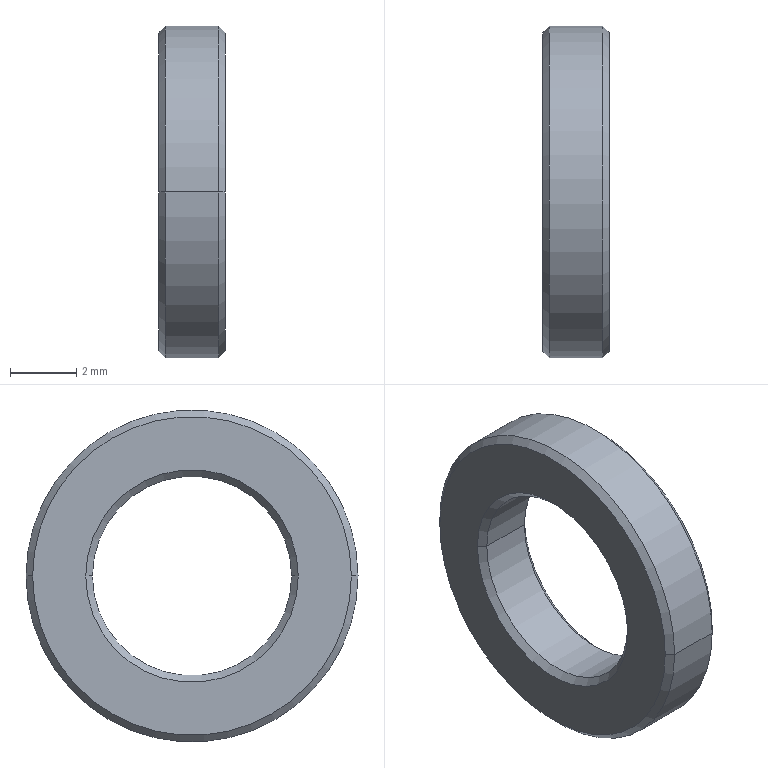Part | STEP file | WSSS10-6-2-32 | 1 solid | 14 faces | box 2 x 10 x 10 mm | volume 98.52 mm3 | cone 8 | cylinder 4 | plane 2 | commonest cylinder face diameters 6 x2 10 x2
STEP:
#1=CARTESIAN_POINT('',(0.,0.,0.));
#2=DIRECTION('',(0.,0.,1.));
#3=DIRECTION('',(1.,0.,0.));
#4=AXIS2_PLACEMENT_3D('',#1,#2,#3);
#5=CARTESIAN_POINT('',(1.8,-3.,0.));
#6=VERTEX_POINT('',#5);
#7=CARTESIAN_POINT('',(0.2,-3.,0.));
#8=VERTEX_POINT('',#7);
#9=CARTESIAN_POINT('',(-3.,-3.,0.));
#10=DIRECTION('',(-1.,0.,0.));
#11=VECTOR('',#10,1.);
#12=LINE('',#9,#11);
#13=CARTESIAN_POINT('',(-3.,0.,0.));
#14=DIRECTION('',(-1.,0.,0.));
#15=DIRECTION('',(0.,-1.,0.));
#16=AXIS2_PLACEMENT_3D('',#13,#14,#15);
#17=CYLINDRICAL_SURFACE('',#16,3.);
#18=CARTESIAN_POINT('',(6.283,0.));
#19=DIRECTION('',(0.,1.));
#20=VECTOR('',#19,1.);
#21=LINE('',#18,#20);
#22=(GEOMETRIC_REPRESENTATION_CONTEXT(2)PARAMETRIC_REPRESENTATION_CONTEXT()REPRESENTATION_CONTEXT('',''));
#23=DEFINITIONAL_REPRESENTATION('',(#21),#22);
#24=PCURVE('',#17,#23);
#25=CARTESIAN_POINT('',(-3.,0.,0.));
#26=DIRECTION('',(-1.,0.,0.));
#27=DIRECTION('',(0.,-1.,0.));
#28=AXIS2_PLACEMENT_3D('',#25,#26,#27);
#29=CYLINDRICAL_SURFACE('',#28,3.);
#30=CARTESIAN_POINT('',(0.,0.));
#31=DIRECTION('',(0.,1.));
#32=VECTOR('',#31,1.);
#33=LINE('',#30,#32);
#34=(GEOMETRIC_REPRESENTATION_CONTEXT(2)PARAMETRIC_REPRESENTATION_CONTEXT()REPRESENTATION_CONTEXT('',''));
#35=DEFINITIONAL_REPRESENTATION('',(#33),#34);
#36=PCURVE('',#29,#35);
#37=SURFACE_CURVE('',#12,(#24,#36),.PCURVE_S1.);
#38=EDGE_CURVE('',#6,#8,#37,.T.);
#39=ORIENTED_EDGE('',*,*,#38,.T.);
#40=CARTESIAN_POINT('',(0.2,3.,0.));
#41=VERTEX_POINT('',#40);
#42=CARTESIAN_POINT('',(0.2,0.,0.));
#43=DIRECTION('',(-1.,0.,0.));
#44=DIRECTION('',(0.,-1.,0.));
#45=AXIS2_PLACEMENT_3D('',#42,#43,#44);
#46=CIRCLE('',#45,3.);
#47=CARTESIAN_POINT('',(0.,-3.2));
#48=DIRECTION('',(1.,0.));
#49=VECTOR('',#48,1.);
#50=LINE('',#47,#49);
#51=(GEOMETRIC_REPRESENTATION_CONTEXT(2)PARAMETRIC_REPRESENTATION_CONTEXT()REPRESENTATION_CONTEXT('',''));
#52=DEFINITIONAL_REPRESENTATION('',(#50),#51);
#53=PCURVE('',#17,#52);
#54=CARTESIAN_POINT('',(0.2,0.,0.));
#55=DIRECTION('',(-1.,0.,0.));
#56=DIRECTION('',(0.,-1.,0.));
#57=AXIS2_PLACEMENT_3D('',#54,#55,#56);
#58=CONICAL_SURFACE('',#57,3.,0.7854);
#59=CARTESIAN_POINT('',(0.,0.));
#60=DIRECTION('',(1.,0.));
#61=VECTOR('',#60,1.);
#62=LINE('',#59,#61);
#63=(GEOMETRIC_REPRESENTATION_CONTEXT(2)PARAMETRIC_REPRESENTATION_CONTEXT()REPRESENTATION_CONTEXT('',''));
#64=DEFINITIONAL_REPRESENTATION('',(#62),#63);
#65=PCURVE('',#58,#64);
#66=SURFACE_CURVE('',#46,(#53,#65),.PCURVE_S1.);
#67=EDGE_CURVE('',#41,#8,#66,.T.);
#68=ORIENTED_EDGE('',*,*,#67,.F.);
#69=CARTESIAN_POINT('',(1.8,3.,0.));
#70=VERTEX_POINT('',#69);
#71=CARTESIAN_POINT('',(-3.,3.,0.));
#72=DIRECTION('',(-1.,0.,0.));
#73=VECTOR('',#72,1.);
#74=LINE('',#71,#73);
#75=CARTESIAN_POINT('',(3.142,0.));
#76=DIRECTION('',(0.,1.));
#77=VECTOR('',#76,1.);
#78=LINE('',#75,#77);
#79=(GEOMETRIC_REPRESENTATION_CONTEXT(2)PARAMETRIC_REPRESENTATION_CONTEXT()REPRESENTATION_CONTEXT('',''));
#80=DEFINITIONAL_REPRESENTATION('',(#78),#79);
#81=PCURVE('',#17,#80);
#82=CARTESIAN_POINT('',(3.142,0.));
#83=DIRECTION('',(0.,1.));
#84=VECTOR('',#83,1.);
#85=LINE('',#82,#84);
#86=(GEOMETRIC_REPRESENTATION_CONTEXT(2)PARAMETRIC_REPRESENTATION_CONTEXT()REPRESENTATION_CONTEXT('',''));
#87=DEFINITIONAL_REPRESENTATION('',(#85),#86);
#88=PCURVE('',#29,#87);
#89=SURFACE_CURVE('',#74,(#81,#88),.PCURVE_S1.);
#90=EDGE_CURVE('',#70,#41,#89,.T.);
#91=ORIENTED_EDGE('',*,*,#90,.F.);
#92=CARTESIAN_POINT('',(1.8,0.,0.));
#93=DIRECTION('',(-1.,0.,0.));
#94=DIRECTION('',(0.,-1.,0.));
#95=AXIS2_PLACEMENT_3D('',#92,#93,#94);
#96=CIRCLE('',#95,3.);
#97=CARTESIAN_POINT('',(0.,-4.8));
#98=DIRECTION('',(1.,0.));
#99=VECTOR('',#98,1.);
#100=LINE('',#97,#99);
#101=(GEOMETRIC_REPRESENTATION_CONTEXT(2)PARAMETRIC_REPRESENTATION_CONTEXT()REPRESENTATION_CONTEXT('',''));
#102=DEFINITIONAL_REPRESENTATION('',(#100),#101);
#103=PCURVE('',#17,#102);
#104=CARTESIAN_POINT('',(2.,0.,0.));
#105=DIRECTION('',(1.,0.,0.));
#106=DIRECTION('',(0.,1.,0.));
#107=AXIS2_PLACEMENT_3D('',#104,#105,#106);
#108=CONICAL_SURFACE('',#107,3.2,0.7854);
#109=CARTESIAN_POINT('',(9.425,-0.2));
#110=DIRECTION('',(-1.,0.));
#111=VECTOR('',#110,1.);
#112=LINE('',#109,#111);
#113=(GEOMETRIC_REPRESENTATION_CONTEXT(2)PARAMETRIC_REPRESENTATION_CONTEXT()REPRESENTATION_CONTEXT('',''));
#114=DEFINITIONAL_REPRESENTATION('',(#112),#113);
#115=PCURVE('',#108,#114);
#116=SURFACE_CURVE('',#96,(#103,#115),.PCURVE_S1.);
#117=EDGE_CURVE('',#70,#6,#116,.T.);
#118=ORIENTED_EDGE('',*,*,#117,.T.);
#119=EDGE_LOOP('',(#39,#68,#91,#118));
#120=FACE_BOUND('',#119,.F.);
#121=ADVANCED_FACE('',(#120),#17,.F.);
#122=CARTESIAN_POINT('',(2.,3.2,0.));
#123=VERTEX_POINT('',#122);
#124=CARTESIAN_POINT('',(2.,3.2,0.));
#125=DIRECTION('',(0.7071,0.7071,0.));
#126=VECTOR('',#125,1.);
#127=LINE('',#124,#126);
#128=CARTESIAN_POINT('',(6.283,0.));
#129=DIRECTION('',(0.,1.));
#130=VECTOR('',#129,1.);
#131=LINE('',#128,#130);
#132=(GEOMETRIC_REPRESENTATION_CONTEXT(2)PARAMETRIC_REPRESENTATION_CONTEXT()REPRESENTATION_CONTEXT('',''));
#133=DEFINITIONAL_REPRESENTATION('',(#131),#132);
#134=PCURVE('',#108,#133);
#135=CARTESIAN_POINT('',(2.,0.,0.));
#136=DIRECTION('',(1.,0.,0.));
#137=DIRECTION('',(0.,1.,0.));
#138=AXIS2_PLACEMENT_3D('',#135,#136,#137);
#139=CONICAL_SURFACE('',#138,3.2,0.7854);
#140=CARTESIAN_POINT('',(0.,0.));
#141=DIRECTION('',(0.,1.));
#142=VECTOR('',#141,1.);
#143=LINE('',#140,#142);
#144=(GEOMETRIC_REPRESENTATION_CONTEXT(2)PARAMETRIC_REPRESENTATION_CONTEXT()REPRESENTATION_CONTEXT('',''));
#145=DEFINITIONAL_REPRESENTATION('',(#143),#144);
#146=PCURVE('',#139,#145);
#147=SURFACE_CURVE('',#127,(#134,#146),.PCURVE_S1.);
#148=EDGE_CURVE('',#70,#123,#147,.T.);
#149=ORIENTED_EDGE('',*,*,#148,.T.);
#150=CARTESIAN_POINT('',(2.,-3.2,0.));
#151=VERTEX_POINT('',#150);
#152=CARTESIAN_POINT('',(2.,0.,0.));
#153=DIRECTION('',(-1.,0.,0.));
#154=DIRECTION('',(0.,-1.,0.));
#155=AXIS2_PLACEMENT_3D('',#152,#153,#154);
#156=CIRCLE('',#155,3.2);
#157=CARTESIAN_POINT('',(9.425,0.));
#158=DIRECTION('',(-1.,0.));
#159=VECTOR('',#158,1.);
#160=LINE('',#157,#159);
#161=(GEOMETRIC_REPRESENTATION_CONTEXT(2)PARAMETRIC_REPRESENTATION_CONTEXT()REPRESENTATION_CONTEXT('',''));
#162=DEFINITIONAL_REPRESENTATION('',(#160),#161);
#163=PCURVE('',#108,#162);
#164=CARTESIAN_POINT('',(2.,-4.8,0.));
#165=DIRECTION('',(1.,0.,0.));
#166=DIRECTION('',(0.,1.,0.));
#167=AXIS2_PLACEMENT_3D('',#164,#165,#166);
#168=PLANE('',#167);
#169=CARTESIAN_POINT('',(1.6,0.));
#170=CARTESIAN_POINT('',(1.6,5.543));
#171=CARTESIAN_POINT('',(6.4,2.771));
#172=CARTESIAN_POINT('',(11.2,0.));
#173=CARTESIAN_POINT('',(6.4,-2.771));
#174=CARTESIAN_POINT('',(1.6,-5.543));
#175=CARTESIAN_POINT('',(1.6,0.));
#176=(BOUNDED_CURVE()B_SPLINE_CURVE(2,(#169,#170,#171,#172,#173,#174,#175),.UNSPECIFIED.,.T.,.F.)B_SPLINE_CURVE_WITH_KNOTS((1,2,2,2,2,1),(-2.094,0.,2.094,4.189,6.283,8.378),.UNSPECIFIED.)CURVE()GEOMETRIC_REPRESENTATION_ITEM()RATIONAL_B_SPLINE_CURVE((1.,0.5,1.,0.5,1.,0.5,1.))REPRESENTATION_ITEM(''));
#177=(GEOMETRIC_REPRESENTATION_CONTEXT(2)PARAMETRIC_REPRESENTATION_CONTEXT()REPRESENTATION_CONTEXT('',''));
#178=DEFINITIONAL_REPRESENTATION('',(#176),#177);
#179=PCURVE('',#168,#178);
#180=SURFACE_CURVE('',#156,(#163,#179),.PCURVE_S1.);
#181=EDGE_CURVE('',#123,#151,#180,.T.);
#182=ORIENTED_EDGE('',*,*,#181,.T.);
#183=CARTESIAN_POINT('',(2.,-3.2,0.));
#184=DIRECTION('',(0.7071,-0.7071,0.));
#185=VECTOR('',#184,1.);
#186=LINE('',#183,#185);
#187=CARTESIAN_POINT('',(3.142,0.));
#188=DIRECTION('',(0.,1.));
#189=VECTOR('',#188,1.);
#190=LINE('',#187,#189);
#191=(GEOMETRIC_REPRESENTATION_CONTEXT(2)PARAMETRIC_REPRESENTATION_CONTEXT()REPRESENTATION_CONTEXT('',''));
#192=DEFINITIONAL_REPRESENTATION('',(#190),#191);
#193=PCURVE('',#108,#192);
#194=CARTESIAN_POINT('',(3.142,0.));
#195=DIRECTION('',(0.,1.));
#196=VECTOR('',#195,1.);
#197=LINE('',#194,#196);
#198=(GEOMETRIC_REPRESENTATION_CONTEXT(2)PARAMETRIC_REPRESENTATION_CONTEXT()REPRESENTATION_CONTEXT('',''));
#199=DEFINITIONAL_REPRESENTATION('',(#197),#198);
#200=PCURVE('',#139,#199);
#201=SURFACE_CURVE('',#186,(#193,#200),.PCURVE_S1.);
#202=EDGE_CURVE('',#6,#151,#201,.T.);
#203=ORIENTED_EDGE('',*,*,#202,.F.);
#204=ORIENTED_EDGE('',*,*,#117,.F.);
#205=EDGE_LOOP('',(#149,#182,#203,#204));
#206=FACE_BOUND('',#205,.F.);
#207=ADVANCED_FACE('',(#206),#108,.F.);
#208=CARTESIAN_POINT('',(2.,-4.8,0.));
#209=VERTEX_POINT('',#208);
#210=CARTESIAN_POINT('',(2.,4.8,0.));
#211=VERTEX_POINT('',#210);
#212=CARTESIAN_POINT('',(2.,0.,0.));
#213=DIRECTION('',(-1.,0.,0.));
#214=DIRECTION('',(0.,-1.,0.));
#215=AXIS2_PLACEMENT_3D('',#212,#213,#214);
#216=CIRCLE('',#215,4.8);
#217=CARTESIAN_POINT('',(1.8,0.,0.));
#218=DIRECTION('',(-1.,0.,0.));
#219=DIRECTION('',(0.,-1.,0.));
#220=AXIS2_PLACEMENT_3D('',#217,#218,#219);
#221=CONICAL_SURFACE('',#220,5.,0.7854);
#222=CARTESIAN_POINT('',(0.,-0.2));
#223=DIRECTION('',(1.,0.));
#224=VECTOR('',#223,1.);
#225=LINE('',#222,#224);
#226=(GEOMETRIC_REPRESENTATION_CONTEXT(2)PARAMETRIC_REPRESENTATION_CONTEXT()REPRESENTATION_CONTEXT('',''));
#227=DEFINITIONAL_REPRESENTATION('',(#225),#226);
#228=PCURVE('',#221,#227);
#229=CARTESIAN_POINT('',(0.,0.));
#230=CARTESIAN_POINT('',(0.,8.314));
#231=CARTESIAN_POINT('',(7.2,4.157));
#232=CARTESIAN_POINT('',(14.4,0.));
#233=CARTESIAN_POINT('',(7.2,-4.157));
#234=CARTESIAN_POINT('',(0.,-8.314));
#235=CARTESIAN_POINT('',(0.,0.));
#236=(BOUNDED_CURVE()B_SPLINE_CURVE(2,(#229,#230,#231,#232,#233,#234,#235),.UNSPECIFIED.,.T.,.F.)B_SPLINE_CURVE_WITH_KNOTS((1,2,2,2,2,1),(-2.094,0.,2.094,4.189,6.283,8.378),.UNSPECIFIED.)CURVE()GEOMETRIC_REPRESENTATION_ITEM()RATIONAL_B_SPLINE_CURVE((1.,0.5,1.,0.5,1.,0.5,1.))REPRESENTATION_ITEM(''));
#237=(GEOMETRIC_REPRESENTATION_CONTEXT(2)PARAMETRIC_REPRESENTATION_CONTEXT()REPRESENTATION_CONTEXT('',''));
#238=DEFINITIONAL_REPRESENTATION('',(#236),#237);
#239=PCURVE('',#168,#238);
#240=SURFACE_CURVE('',#216,(#228,#239),.PCURVE_S1.);
#241=EDGE_CURVE('',#209,#211,#240,.T.);
#242=ORIENTED_EDGE('',*,*,#241,.T.);
#243=CARTESIAN_POINT('',(1.8,5.,0.));
#244=VERTEX_POINT('',#243);
#245=CARTESIAN_POINT('',(1.8,5.,0.));
#246=DIRECTION('',(-0.7071,0.7071,0.));
#247=VECTOR('',#246,1.);
#248=LINE('',#245,#247);
#249=CARTESIAN_POINT('',(3.142,0.));
#250=DIRECTION('',(0.,1.));
#251=VECTOR('',#250,1.);
#252=LINE('',#249,#251);
#253=(GEOMETRIC_REPRESENTATION_CONTEXT(2)PARAMETRIC_REPRESENTATION_CONTEXT()REPRESENTATION_CONTEXT('',''));
#254=DEFINITIONAL_REPRESENTATION('',(#252),#253);
#255=PCURVE('',#221,#254);
#256=CARTESIAN_POINT('',(1.8,0.,0.));
#257=DIRECTION('',(-1.,0.,0.));
#258=DIRECTION('',(0.,-1.,0.));
#259=AXIS2_PLACEMENT_3D('',#256,#257,#258);
#260=CONICAL_SURFACE('',#259,5.,0.7854);
#261=CARTESIAN_POINT('',(3.142,0.));
#262=DIRECTION('',(0.,1.));
#263=VECTOR('',#262,1.);
#264=LINE('',#261,#263);
#265=(GEOMETRIC_REPRESENTATION_CONTEXT(2)PARAMETRIC_REPRESENTATION_CONTEXT()REPRESENTATION_CONTEXT('',''));
#266=DEFINITIONAL_REPRESENTATION('',(#264),#265);
#267=PCURVE('',#260,#266);
#268=SURFACE_CURVE('',#248,(#255,#267),.PCURVE_S1.);
#269=EDGE_CURVE('',#211,#244,#268,.T.);
#270=ORIENTED_EDGE('',*,*,#269,.T.);
#271=CARTESIAN_POINT('',(1.8,-5.,0.));
#272=VERTEX_POINT('',#271);
#273=CARTESIAN_POINT('',(1.8,0.,0.));
#274=DIRECTION('',(-1.,0.,0.));
#275=DIRECTION('',(0.,-1.,0.));
#276=AXIS2_PLACEMENT_3D('',#273,#274,#275);
#277=CIRCLE('',#276,5.);
#278=CARTESIAN_POINT('',(0.,0.));
#279=DIRECTION('',(1.,0.));
#280=VECTOR('',#279,1.);
#281=LINE('',#278,#280);
#282=(GEOMETRIC_REPRESENTATION_CONTEXT(2)PARAMETRIC_REPRESENTATION_CONTEXT()REPRESENTATION_CONTEXT('',''));
#283=DEFINITIONAL_REPRESENTATION('',(#281),#282);
#284=PCURVE('',#221,#283);
#285=CARTESIAN_POINT('',(-3.,0.,0.));
#286=DIRECTION('',(-1.,0.,0.));
#287=DIRECTION('',(0.,-1.,0.));
#288=AXIS2_PLACEMENT_3D('',#285,#286,#287);
#289=CYLINDRICAL_SURFACE('',#288,5.);
#290=CARTESIAN_POINT('',(0.,-4.8));
#291=DIRECTION('',(1.,0.));
#292=VECTOR('',#291,1.);
#293=LINE('',#290,#292);
#294=(GEOMETRIC_REPRESENTATION_CONTEXT(2)PARAMETRIC_REPRESENTATION_CONTEXT()REPRESENTATION_CONTEXT('',''));
#295=DEFINITIONAL_REPRESENTATION('',(#293),#294);
#296=PCURVE('',#289,#295);
#297=SURFACE_CURVE('',#277,(#284,#296),.PCURVE_S1.);
#298=EDGE_CURVE('',#272,#244,#297,.T.);
#299=ORIENTED_EDGE('',*,*,#298,.F.);
#300=CARTESIAN_POINT('',(1.8,-5.,0.));
#301=DIRECTION('',(-0.7071,-0.7071,0.));
#302=VECTOR('',#301,1.);
#303=LINE('',#300,#302);
#304=CARTESIAN_POINT('',(0.,0.));
#305=DIRECTION('',(0.,1.));
#306=VECTOR('',#305,1.);
#307=LINE('',#304,#306);
#308=(GEOMETRIC_REPRESENTATION_CONTEXT(2)PARAMETRIC_REPRESENTATION_CONTEXT()REPRESENTATION_CONTEXT('',''));
#309=DEFINITIONAL_REPRESENTATION('',(#307),#308);
#310=PCURVE('',#221,#309);
#311=CARTESIAN_POINT('',(6.283,0.));
#312=DIRECTION('',(0.,1.));
#313=VECTOR('',#312,1.);
#314=LINE('',#311,#313);
#315=(GEOMETRIC_REPRESENTATION_CONTEXT(2)PARAMETRIC_REPRESENTATION_CONTEXT()REPRESENTATION_CONTEXT('',''));
#316=DEFINITIONAL_REPRESENTATION('',(#314),#315);
#317=PCURVE('',#260,#316);
#318=SURFACE_CURVE('',#303,(#310,#317),.PCURVE_S1.);
#319=EDGE_CURVE('',#209,#272,#318,.T.);
#320=ORIENTED_EDGE('',*,*,#319,.F.);
#321=EDGE_LOOP('',(#242,#270,#299,#320));
#322=FACE_BOUND('',#321,.T.);
#323=ADVANCED_FACE('',(#322),#221,.T.);
#324=ORIENTED_EDGE('',*,*,#298,.T.);
#325=CARTESIAN_POINT('',(0.2,5.,0.));
#326=VERTEX_POINT('',#325);
#327=CARTESIAN_POINT('',(-3.,5.,0.));
#328=DIRECTION('',(-1.,0.,0.));
#329=VECTOR('',#328,1.);
#330=LINE('',#327,#329);
#331=CARTESIAN_POINT('',(3.142,0.));
#332=DIRECTION('',(0.,1.));
#333=VECTOR('',#332,1.);
#334=LINE('',#331,#333);
#335=(GEOMETRIC_REPRESENTATION_CONTEXT(2)PARAMETRIC_REPRESENTATION_CONTEXT()REPRESENTATION_CONTEXT('',''));
#336=DEFINITIONAL_REPRESENTATION('',(#334),#335);
#337=PCURVE('',#289,#336);
#338=CARTESIAN_POINT('',(-3.,0.,0.));
#339=DIRECTION('',(-1.,0.,0.));
#340=DIRECTION('',(0.,-1.,0.));
#341=AXIS2_PLACEMENT_3D('',#338,#339,#340);
#342=CYLINDRICAL_SURFACE('',#341,5.);
#343=CARTESIAN_POINT('',(3.142,0.));
#344=DIRECTION('',(0.,1.));
#345=VECTOR('',#344,1.);
#346=LINE('',#343,#345);
#347=(GEOMETRIC_REPRESENTATION_CONTEXT(2)PARAMETRIC_REPRESENTATION_CONTEXT()REPRESENTATION_CONTEXT('',''));
#348=DEFINITIONAL_REPRESENTATION('',(#346),#347);
#349=PCURVE('',#342,#348);
#350=SURFACE_CURVE('',#330,(#337,#349),.PCURVE_S1.);
#351=EDGE_CURVE('',#244,#326,#350,.T.);
#352=ORIENTED_EDGE('',*,*,#351,.T.);
#353=CARTESIAN_POINT('',(0.2,-5.,0.));
#354=VERTEX_POINT('',#353);
#355=CARTESIAN_POINT('',(0.2,0.,0.));
#356=DIRECTION('',(-1.,0.,0.));
#357=DIRECTION('',(0.,-1.,0.));
#358=AXIS2_PLACEMENT_3D('',#355,#356,#357);
#359=CIRCLE('',#358,5.);
#360=CARTESIAN_POINT('',(0.,-3.2));
#361=DIRECTION('',(1.,0.));
#362=VECTOR('',#361,1.);
#363=LINE('',#360,#362);
#364=(GEOMETRIC_REPRESENTATION_CONTEXT(2)PARAMETRIC_REPRESENTATION_CONTEXT()REPRESENTATION_CONTEXT('',''));
#365=DEFINITIONAL_REPRESENTATION('',(#363),#364);
#366=PCURVE('',#289,#365);
#367=CARTESIAN_POINT('',(0.,0.,0.));
#368=DIRECTION('',(1.,0.,0.));
#369=DIRECTION('',(0.,1.,0.));
#370=AXIS2_PLACEMENT_3D('',#367,#368,#369);
#371=CONICAL_SURFACE('',#370,4.8,0.7854);
#372=CARTESIAN_POINT('',(3.142,0.2));
#373=DIRECTION('',(-1.,0.));
#374=VECTOR('',#373,1.);
#375=LINE('',#372,#374);
#376=(GEOMETRIC_REPRESENTATION_CONTEXT(2)PARAMETRIC_REPRESENTATION_CONTEXT()REPRESENTATION_CONTEXT('',''));
#377=DEFINITIONAL_REPRESENTATION('',(#375),#376);
#378=PCURVE('',#371,#377);
#379=SURFACE_CURVE('',#359,(#366,#378),.PCURVE_S1.);
#380=EDGE_CURVE('',#354,#326,#379,.T.);
#381=ORIENTED_EDGE('',*,*,#380,.F.);
#382=CARTESIAN_POINT('',(-3.,-5.,0.));
#383=DIRECTION('',(-1.,0.,0.));
#384=VECTOR('',#383,1.);
#385=LINE('',#382,#384);
#386=CARTESIAN_POINT('',(0.,0.));
#387=DIRECTION('',(0.,1.));
#388=VECTOR('',#387,1.);
#389=LINE('',#386,#388);
#390=(GEOMETRIC_REPRESENTATION_CONTEXT(2)PARAMETRIC_REPRESENTATION_CONTEXT()REPRESENTATION_CONTEXT('',''));
#391=DEFINITIONAL_REPRESENTATION('',(#389),#390);
#392=PCURVE('',#289,#391);
#393=CARTESIAN_POINT('',(6.283,0.));
#394=DIRECTION('',(0.,1.));
#395=VECTOR('',#394,1.);
#396=LINE('',#393,#395);
#397=(GEOMETRIC_REPRESENTATION_CONTEXT(2)PARAMETRIC_REPRESENTATION_CONTEXT()REPRESENTATION_CONTEXT('',''));
#398=DEFINITIONAL_REPRESENTATION('',(#396),#397);
#399=PCURVE('',#342,#398);
#400=SURFACE_CURVE('',#385,(#392,#399),.PCURVE_S1.);
#401=EDGE_CURVE('',#272,#354,#400,.T.);
#402=ORIENTED_EDGE('',*,*,#401,.F.);
#403=EDGE_LOOP('',(#324,#352,#381,#402));
#404=FACE_BOUND('',#403,.T.);
#405=ADVANCED_FACE('',(#404),#289,.T.);
#406=CARTESIAN_POINT('',(0.,-4.8,0.));
#407=VERTEX_POINT('',#406);
#408=CARTESIAN_POINT('',(0.,4.8,0.));
#409=VERTEX_POINT('',#408);
#410=CARTESIAN_POINT('',(0.,0.,0.));
#411=DIRECTION('',(-1.,0.,0.));
#412=DIRECTION('',(0.,-1.,0.));
#413=AXIS2_PLACEMENT_3D('',#410,#411,#412);
#414=CIRCLE('',#413,4.8);
#415=CARTESIAN_POINT('',(3.142,0.));
#416=DIRECTION('',(-1.,0.));
#417=VECTOR('',#416,1.);
#418=LINE('',#415,#417);
#419=(GEOMETRIC_REPRESENTATION_CONTEXT(2)PARAMETRIC_REPRESENTATION_CONTEXT()REPRESENTATION_CONTEXT('',''));
#420=DEFINITIONAL_REPRESENTATION('',(#418),#419);
#421=PCURVE('',#371,#420);
#422=CARTESIAN_POINT('',(0.,-3.2,0.));
#423=DIRECTION('',(-1.,0.,0.));
#424=DIRECTION('',(0.,-1.,0.));
#425=AXIS2_PLACEMENT_3D('',#422,#423,#424);
#426=PLANE('',#425);
#427=CARTESIAN_POINT('',(-3.2,0.));
#428=DIRECTION('',(1.,0.));
#429=AXIS2_PLACEMENT_2D('',#427,#428);
#430=CIRCLE('',#429,4.8);
#431=(GEOMETRIC_REPRESENTATION_CONTEXT(2)PARAMETRIC_REPRESENTATION_CONTEXT()REPRESENTATION_CONTEXT('',''));
#432=DEFINITIONAL_REPRESENTATION('',(#430),#431);
#433=PCURVE('',#426,#432);
#434=SURFACE_CURVE('',#414,(#421,#433),.PCURVE_S1.);
#435=EDGE_CURVE('',#407,#409,#434,.T.);
#436=ORIENTED_EDGE('',*,*,#435,.F.);
#437=CARTESIAN_POINT('',(0.,-4.8,0.));
#438=DIRECTION('',(0.7071,-0.7071,0.));
#439=VECTOR('',#438,1.);
#440=LINE('',#437,#439);
#441=CARTESIAN_POINT('',(3.142,0.));
#442=DIRECTION('',(0.,1.));
#443=VECTOR('',#442,1.);
#444=LINE('',#441,#443);
#445=(GEOMETRIC_REPRESENTATION_CONTEXT(2)PARAMETRIC_REPRESENTATION_CONTEXT()REPRESENTATION_CONTEXT('',''));
#446=DEFINITIONAL_REPRESENTATION('',(#444),#445);
#447=PCURVE('',#371,#446);
#448=CARTESIAN_POINT('',(0.,0.,0.));
#449=DIRECTION('',(1.,0.,0.));
#450=DIRECTION('',(0.,1.,0.));
#451=AXIS2_PLACEMENT_3D('',#448,#449,#450);
#452=CONICAL_SURFACE('',#451,4.8,0.7854);
#453=CARTESIAN_POINT('',(3.142,0.));
#454=DIRECTION('',(0.,1.));
#455=VECTOR('',#454,1.);
#456=LINE('',#453,#455);
#457=(GEOMETRIC_REPRESENTATION_CONTEXT(2)PARAMETRIC_REPRESENTATION_CONTEXT()REPRESENTATION_CONTEXT('',''));
#458=DEFINITIONAL_REPRESENTATION('',(#456),#457);
#459=PCURVE('',#452,#458);
#460=SURFACE_CURVE('',#440,(#447,#459),.PCURVE_S1.);
#461=EDGE_CURVE('',#407,#354,#460,.T.);
#462=ORIENTED_EDGE('',*,*,#461,.T.);
#463=ORIENTED_EDGE('',*,*,#380,.T.);
#464=CARTESIAN_POINT('',(0.,4.8,0.));
#465=DIRECTION('',(0.7071,0.7071,0.));
#466=VECTOR('',#465,1.);
#467=LINE('',#464,#466);
#468=CARTESIAN_POINT('',(0.,0.));
#469=DIRECTION('',(0.,1.));
#470=VECTOR('',#469,1.);
#471=LINE('',#468,#470);
#472=(GEOMETRIC_REPRESENTATION_CONTEXT(2)PARAMETRIC_REPRESENTATION_CONTEXT()REPRESENTATION_CONTEXT('',''));
#473=DEFINITIONAL_REPRESENTATION('',(#471),#472);
#474=PCURVE('',#371,#473);
#475=CARTESIAN_POINT('',(6.283,0.));
#476=DIRECTION('',(0.,1.));
#477=VECTOR('',#476,1.);
#478=LINE('',#475,#477);
#479=(GEOMETRIC_REPRESENTATION_CONTEXT(2)PARAMETRIC_REPRESENTATION_CONTEXT()REPRESENTATION_CONTEXT('',''));
#480=DEFINITIONAL_REPRESENTATION('',(#478),#479);
#481=PCURVE('',#452,#480);
#482=SURFACE_CURVE('',#467,(#474,#481),.PCURVE_S1.);
#483=EDGE_CURVE('',#409,#326,#482,.T.);
#484=ORIENTED_EDGE('',*,*,#483,.F.);
#485=EDGE_LOOP('',(#436,#462,#463,#484));
#486=FACE_BOUND('',#485,.T.);
#487=ADVANCED_FACE('',(#486),#371,.T.);
#488=CARTESIAN_POINT('',(0.,-3.2,0.));
#489=VERTEX_POINT('',#488);
#490=CARTESIAN_POINT('',(0.2,-3.,0.));
#491=DIRECTION('',(-0.7071,-0.7071,0.));
#492=VECTOR('',#491,1.);
#493=LINE('',#490,#492);
#494=CARTESIAN_POINT('',(6.283,0.));
#495=DIRECTION('',(0.,1.));
#496=VECTOR('',#495,1.);
#497=LINE('',#494,#496);
#498=(GEOMETRIC_REPRESENTATION_CONTEXT(2)PARAMETRIC_REPRESENTATION_CONTEXT()REPRESENTATION_CONTEXT('',''));
#499=DEFINITIONAL_REPRESENTATION('',(#497),#498);
#500=PCURVE('',#58,#499);
#501=CARTESIAN_POINT('',(0.2,0.,0.));
#502=DIRECTION('',(-1.,0.,0.));
#503=DIRECTION('',(0.,-1.,0.));
#504=AXIS2_PLACEMENT_3D('',#501,#502,#503);
#505=CONICAL_SURFACE('',#504,3.,0.7854);
#506=CARTESIAN_POINT('',(0.,0.));
#507=DIRECTION('',(0.,1.));
#508=VECTOR('',#507,1.);
#509=LINE('',#506,#508);
#510=(GEOMETRIC_REPRESENTATION_CONTEXT(2)PARAMETRIC_REPRESENTATION_CONTEXT()REPRESENTATION_CONTEXT('',''));
#511=DEFINITIONAL_REPRESENTATION('',(#509),#510);
#512=PCURVE('',#505,#511);
#513=SURFACE_CURVE('',#493,(#500,#512),.PCURVE_S1.);
#514=EDGE_CURVE('',#8,#489,#513,.T.);
#515=ORIENTED_EDGE('',*,*,#514,.T.);
#516=CARTESIAN_POINT('',(0.,3.2,0.));
#517=VERTEX_POINT('',#516);
#518=CARTESIAN_POINT('',(0.,0.,0.));
#519=DIRECTION('',(-1.,0.,0.));
#520=DIRECTION('',(0.,-1.,0.));
#521=AXIS2_PLACEMENT_3D('',#518,#519,#520);
#522=CIRCLE('',#521,3.2);
#523=CARTESIAN_POINT('',(0.,0.2));
#524=DIRECTION('',(1.,0.));
#525=VECTOR('',#524,1.);
#526=LINE('',#523,#525);
#527=(GEOMETRIC_REPRESENTATION_CONTEXT(2)PARAMETRIC_REPRESENTATION_CONTEXT()REPRESENTATION_CONTEXT('',''));
#528=DEFINITIONAL_REPRESENTATION('',(#526),#527);
#529=PCURVE('',#58,#528);
#530=CARTESIAN_POINT('',(-3.2,0.));
#531=DIRECTION('',(1.,0.));
#532=AXIS2_PLACEMENT_2D('',#530,#531);
#533=CIRCLE('',#532,3.2);
#534=(GEOMETRIC_REPRESENTATION_CONTEXT(2)PARAMETRIC_REPRESENTATION_CONTEXT()REPRESENTATION_CONTEXT('',''));
#535=DEFINITIONAL_REPRESENTATION('',(#533),#534);
#536=PCURVE('',#426,#535);
#537=SURFACE_CURVE('',#522,(#529,#536),.PCURVE_S1.);
#538=EDGE_CURVE('',#517,#489,#537,.T.);
#539=ORIENTED_EDGE('',*,*,#538,.F.);
#540=CARTESIAN_POINT('',(0.2,3.,0.));
#541=DIRECTION('',(-0.7071,0.7071,0.));
#542=VECTOR('',#541,1.);
#543=LINE('',#540,#542);
#544=CARTESIAN_POINT('',(3.142,0.));
#545=DIRECTION('',(0.,1.));
#546=VECTOR('',#545,1.);
#547=LINE('',#544,#546);
#548=(GEOMETRIC_REPRESENTATION_CONTEXT(2)PARAMETRIC_REPRESENTATION_CONTEXT()REPRESENTATION_CONTEXT('',''));
#549=DEFINITIONAL_REPRESENTATION('',(#547),#548);
#550=PCURVE('',#58,#549);
#551=CARTESIAN_POINT('',(3.142,0.));
#552=DIRECTION('',(0.,1.));
#553=VECTOR('',#552,1.);
#554=LINE('',#551,#553);
#555=(GEOMETRIC_REPRESENTATION_CONTEXT(2)PARAMETRIC_REPRESENTATION_CONTEXT()REPRESENTATION_CONTEXT('',''));
#556=DEFINITIONAL_REPRESENTATION('',(#554),#555);
#557=PCURVE('',#505,#556);
#558=SURFACE_CURVE('',#543,(#550,#557),.PCURVE_S1.);
#559=EDGE_CURVE('',#41,#517,#558,.T.);
#560=ORIENTED_EDGE('',*,*,#559,.F.);
#561=ORIENTED_EDGE('',*,*,#67,.T.);
#562=EDGE_LOOP('',(#515,#539,#560,#561));
#563=FACE_BOUND('',#562,.F.);
#564=ADVANCED_FACE('',(#563),#58,.F.);
#565=CARTESIAN_POINT('',(0.,0.,0.));
#566=DIRECTION('',(-1.,0.,0.));
#567=DIRECTION('',(0.,-1.,0.));
#568=AXIS2_PLACEMENT_3D('',#565,#566,#567);
#569=CIRCLE('',#568,3.2);
#570=CARTESIAN_POINT('',(0.,0.2));
#571=DIRECTION('',(1.,0.));
#572=VECTOR('',#571,1.);
#573=LINE('',#570,#572);
#574=(GEOMETRIC_REPRESENTATION_CONTEXT(2)PARAMETRIC_REPRESENTATION_CONTEXT()REPRESENTATION_CONTEXT('',''));
#575=DEFINITIONAL_REPRESENTATION('',(#573),#574);
#576=PCURVE('',#505,#575);
#577=CARTESIAN_POINT('',(-3.2,0.));
#578=DIRECTION('',(1.,0.));
#579=AXIS2_PLACEMENT_2D('',#577,#578);
#580=CIRCLE('',#579,3.2);
#581=(GEOMETRIC_REPRESENTATION_CONTEXT(2)PARAMETRIC_REPRESENTATION_CONTEXT()REPRESENTATION_CONTEXT('',''));
#582=DEFINITIONAL_REPRESENTATION('',(#580),#581);
#583=PCURVE('',#426,#582);
#584=SURFACE_CURVE('',#569,(#576,#583),.PCURVE_S1.);
#585=EDGE_CURVE('',#489,#517,#584,.T.);
#586=ORIENTED_EDGE('',*,*,#585,.F.);
#587=ORIENTED_EDGE('',*,*,#514,.F.);
#588=CARTESIAN_POINT('',(0.2,0.,0.));
#589=DIRECTION('',(-1.,0.,0.));
#590=DIRECTION('',(0.,-1.,0.));
#591=AXIS2_PLACEMENT_3D('',#588,#589,#590);
#592=CIRCLE('',#591,3.);
#593=CARTESIAN_POINT('',(0.,0.));
#594=DIRECTION('',(1.,0.));
#595=VECTOR('',#594,1.);
#596=LINE('',#593,#595);
#597=(GEOMETRIC_REPRESENTATION_CONTEXT(2)PARAMETRIC_REPRESENTATION_CONTEXT()REPRESENTATION_CONTEXT('',''));
#598=DEFINITIONAL_REPRESENTATION('',(#596),#597);
#599=PCURVE('',#505,#598);
#600=CARTESIAN_POINT('',(0.,-3.2));
#601=DIRECTION('',(1.,0.));
#602=VECTOR('',#601,1.);
#603=LINE('',#600,#602);
#604=(GEOMETRIC_REPRESENTATION_CONTEXT(2)PARAMETRIC_REPRESENTATION_CONTEXT()REPRESENTATION_CONTEXT('',''));
#605=DEFINITIONAL_REPRESENTATION('',(#603),#604);
#606=PCURVE('',#29,#605);
#607=SURFACE_CURVE('',#592,(#599,#606),.PCURVE_S1.);
#608=EDGE_CURVE('',#8,#41,#607,.T.);
#609=ORIENTED_EDGE('',*,*,#608,.T.);
#610=ORIENTED_EDGE('',*,*,#559,.T.);
#611=EDGE_LOOP('',(#586,#587,#609,#610));
#612=FACE_BOUND('',#611,.F.);
#613=ADVANCED_FACE('',(#612),#505,.F.);
#614=CARTESIAN_POINT('',(0.,0.,0.));
#615=DIRECTION('',(-1.,0.,0.));
#616=DIRECTION('',(0.,-1.,0.));
#617=AXIS2_PLACEMENT_3D('',#614,#615,#616);
#618=CIRCLE('',#617,4.8);
#619=CARTESIAN_POINT('',(-3.2,0.));
#620=DIRECTION('',(1.,0.));
#621=AXIS2_PLACEMENT_2D('',#619,#620);
#622=CIRCLE('',#621,4.8);
#623=(GEOMETRIC_REPRESENTATION_CONTEXT(2)PARAMETRIC_REPRESENTATION_CONTEXT()REPRESENTATION_CONTEXT('',''));
#624=DEFINITIONAL_REPRESENTATION('',(#622),#623);
#625=PCURVE('',#426,#624);
#626=CARTESIAN_POINT('',(9.425,0.));
#627=DIRECTION('',(-1.,0.));
#628=VECTOR('',#627,1.);
#629=LINE('',#626,#628);
#630=(GEOMETRIC_REPRESENTATION_CONTEXT(2)PARAMETRIC_REPRESENTATION_CONTEXT()REPRESENTATION_CONTEXT('',''));
#631=DEFINITIONAL_REPRESENTATION('',(#629),#630);
#632=PCURVE('',#452,#631);
#633=SURFACE_CURVE('',#618,(#625,#632),.PCURVE_S1.);
#634=EDGE_CURVE('',#409,#407,#633,.T.);
#635=ORIENTED_EDGE('',*,*,#634,.T.);
#636=ORIENTED_EDGE('',*,*,#435,.T.);
#637=EDGE_LOOP('',(#635,#636));
#638=FACE_BOUND('',#637,.T.);
#639=ORIENTED_EDGE('',*,*,#585,.F.);
#640=ORIENTED_EDGE('',*,*,#538,.F.);
#641=EDGE_LOOP('',(#639,#640));
#642=FACE_BOUND('',#641,.T.);
#643=ADVANCED_FACE('',(#638,#642),#426,.T.);
#644=ORIENTED_EDGE('',*,*,#461,.F.);
#645=ORIENTED_EDGE('',*,*,#634,.F.);
#646=ORIENTED_EDGE('',*,*,#483,.T.);
#647=CARTESIAN_POINT('',(0.2,0.,0.));
#648=DIRECTION('',(-1.,0.,0.));
#649=DIRECTION('',(0.,-1.,0.));
#650=AXIS2_PLACEMENT_3D('',#647,#648,#649);
#651=CIRCLE('',#650,5.);
#652=CARTESIAN_POINT('',(9.425,0.2));
#653=DIRECTION('',(-1.,0.));
#654=VECTOR('',#653,1.);
#655=LINE('',#652,#654);
#656=(GEOMETRIC_REPRESENTATION_CONTEXT(2)PARAMETRIC_REPRESENTATION_CONTEXT()REPRESENTATION_CONTEXT('',''));
#657=DEFINITIONAL_REPRESENTATION('',(#655),#656);
#658=PCURVE('',#452,#657);
#659=CARTESIAN_POINT('',(0.,-3.2));
#660=DIRECTION('',(1.,0.));
#661=VECTOR('',#660,1.);
#662=LINE('',#659,#661);
#663=(GEOMETRIC_REPRESENTATION_CONTEXT(2)PARAMETRIC_REPRESENTATION_CONTEXT()REPRESENTATION_CONTEXT('',''));
#664=DEFINITIONAL_REPRESENTATION('',(#662),#663);
#665=PCURVE('',#342,#664);
#666=SURFACE_CURVE('',#651,(#658,#665),.PCURVE_S1.);
#667=EDGE_CURVE('',#326,#354,#666,.T.);
#668=ORIENTED_EDGE('',*,*,#667,.T.);
#669=EDGE_LOOP('',(#644,#645,#646,#668));
#670=FACE_BOUND('',#669,.T.);
#671=ADVANCED_FACE('',(#670),#452,.T.);
#672=ORIENTED_EDGE('',*,*,#351,.F.);
#673=CARTESIAN_POINT('',(1.8,0.,0.));
#674=DIRECTION('',(-1.,0.,0.));
#675=DIRECTION('',(0.,-1.,0.));
#676=AXIS2_PLACEMENT_3D('',#673,#674,#675);
#677=CIRCLE('',#676,5.);
#678=CARTESIAN_POINT('',(0.,-4.8));
#679=DIRECTION('',(1.,0.));
#680=VECTOR('',#679,1.);
#681=LINE('',#678,#680);
#682=(GEOMETRIC_REPRESENTATION_CONTEXT(2)PARAMETRIC_REPRESENTATION_CONTEXT()REPRESENTATION_CONTEXT('',''));
#683=DEFINITIONAL_REPRESENTATION('',(#681),#682);
#684=PCURVE('',#342,#683);
#685=CARTESIAN_POINT('',(0.,0.));
#686=DIRECTION('',(1.,0.));
#687=VECTOR('',#686,1.);
#688=LINE('',#685,#687);
#689=(GEOMETRIC_REPRESENTATION_CONTEXT(2)PARAMETRIC_REPRESENTATION_CONTEXT()REPRESENTATION_CONTEXT('',''));
#690=DEFINITIONAL_REPRESENTATION('',(#688),#689);
#691=PCURVE('',#260,#690);
#692=SURFACE_CURVE('',#677,(#684,#691),.PCURVE_S1.);
#693=EDGE_CURVE('',#244,#272,#692,.T.);
#694=ORIENTED_EDGE('',*,*,#693,.T.);
#695=ORIENTED_EDGE('',*,*,#401,.T.);
#696=ORIENTED_EDGE('',*,*,#667,.F.);
#697=EDGE_LOOP('',(#672,#694,#695,#696));
#698=FACE_BOUND('',#697,.T.);
#699=ADVANCED_FACE('',(#698),#342,.T.);
#700=ORIENTED_EDGE('',*,*,#269,.F.);
#701=CARTESIAN_POINT('',(2.,0.,0.));
#702=DIRECTION('',(-1.,0.,0.));
#703=DIRECTION('',(0.,-1.,0.));
#704=AXIS2_PLACEMENT_3D('',#701,#702,#703);
#705=CIRCLE('',#704,4.8);
#706=CARTESIAN_POINT('',(0.,-0.2));
#707=DIRECTION('',(1.,0.));
#708=VECTOR('',#707,1.);
#709=LINE('',#706,#708);
#710=(GEOMETRIC_REPRESENTATION_CONTEXT(2)PARAMETRIC_REPRESENTATION_CONTEXT()REPRESENTATION_CONTEXT('',''));
#711=DEFINITIONAL_REPRESENTATION('',(#709),#710);
#712=PCURVE('',#260,#711);
#713=CARTESIAN_POINT('',(0.,0.));
#714=CARTESIAN_POINT('',(0.,8.314));
#715=CARTESIAN_POINT('',(7.2,4.157));
#716=CARTESIAN_POINT('',(14.4,0.));
#717=CARTESIAN_POINT('',(7.2,-4.157));
#718=CARTESIAN_POINT('',(0.,-8.314));
#719=CARTESIAN_POINT('',(0.,0.));
#720=(BOUNDED_CURVE()B_SPLINE_CURVE(2,(#713,#714,#715,#716,#717,#718,#719),.UNSPECIFIED.,.T.,.F.)B_SPLINE_CURVE_WITH_KNOTS((1,2,2,2,2,1),(-2.094,0.,2.094,4.189,6.283,8.378),.UNSPECIFIED.)CURVE()GEOMETRIC_REPRESENTATION_ITEM()RATIONAL_B_SPLINE_CURVE((1.,0.5,1.,0.5,1.,0.5,1.))REPRESENTATION_ITEM(''));
#721=(GEOMETRIC_REPRESENTATION_CONTEXT(2)PARAMETRIC_REPRESENTATION_CONTEXT()REPRESENTATION_CONTEXT('',''));
#722=DEFINITIONAL_REPRESENTATION('',(#720),#721);
#723=PCURVE('',#168,#722);
#724=SURFACE_CURVE('',#705,(#712,#723),.PCURVE_S1.);
#725=EDGE_CURVE('',#211,#209,#724,.T.);
#726=ORIENTED_EDGE('',*,*,#725,.T.);
#727=ORIENTED_EDGE('',*,*,#319,.T.);
#728=ORIENTED_EDGE('',*,*,#693,.F.);
#729=EDGE_LOOP('',(#700,#726,#727,#728));
#730=FACE_BOUND('',#729,.T.);
#731=ADVANCED_FACE('',(#730),#260,.T.);
#732=ORIENTED_EDGE('',*,*,#181,.T.);
#733=CARTESIAN_POINT('',(2.,0.,0.));
#734=DIRECTION('',(-1.,0.,0.));
#735=DIRECTION('',(0.,-1.,0.));
#736=AXIS2_PLACEMENT_3D('',#733,#734,#735);
#737=CIRCLE('',#736,3.2);
#738=CARTESIAN_POINT('',(1.6,0.));
#739=CARTESIAN_POINT('',(1.6,5.543));
#740=CARTESIAN_POINT('',(6.4,2.771));
#741=CARTESIAN_POINT('',(11.2,0.));
#742=CARTESIAN_POINT('',(6.4,-2.771));
#743=CARTESIAN_POINT('',(1.6,-5.543));
#744=CARTESIAN_POINT('',(1.6,0.));
#745=(BOUNDED_CURVE()B_SPLINE_CURVE(2,(#738,#739,#740,#741,#742,#743,#744),.UNSPECIFIED.,.T.,.F.)B_SPLINE_CURVE_WITH_KNOTS((1,2,2,2,2,1),(-2.094,0.,2.094,4.189,6.283,8.378),.UNSPECIFIED.)CURVE()GEOMETRIC_REPRESENTATION_ITEM()RATIONAL_B_SPLINE_CURVE((1.,0.5,1.,0.5,1.,0.5,1.))REPRESENTATION_ITEM(''));
#746=(GEOMETRIC_REPRESENTATION_CONTEXT(2)PARAMETRIC_REPRESENTATION_CONTEXT()REPRESENTATION_CONTEXT('',''));
#747=DEFINITIONAL_REPRESENTATION('',(#745),#746);
#748=PCURVE('',#168,#747);
#749=CARTESIAN_POINT('',(3.142,0.));
#750=DIRECTION('',(-1.,0.));
#751=VECTOR('',#750,1.);
#752=LINE('',#749,#751);
#753=(GEOMETRIC_REPRESENTATION_CONTEXT(2)PARAMETRIC_REPRESENTATION_CONTEXT()REPRESENTATION_CONTEXT('',''));
#754=DEFINITIONAL_REPRESENTATION('',(#752),#753);
#755=PCURVE('',#139,#754);
#756=SURFACE_CURVE('',#737,(#748,#755),.PCURVE_S1.);
#757=EDGE_CURVE('',#151,#123,#756,.T.);
#758=ORIENTED_EDGE('',*,*,#757,.T.);
#759=EDGE_LOOP('',(#732,#758));
#760=FACE_BOUND('',#759,.T.);
#761=ORIENTED_EDGE('',*,*,#241,.F.);
#762=ORIENTED_EDGE('',*,*,#725,.F.);
#763=EDGE_LOOP('',(#761,#762));
#764=FACE_BOUND('',#763,.T.);
#765=ADVANCED_FACE('',(#760,#764),#168,.T.);
#766=ORIENTED_EDGE('',*,*,#757,.T.);
#767=ORIENTED_EDGE('',*,*,#148,.F.);
#768=CARTESIAN_POINT('',(1.8,0.,0.));
#769=DIRECTION('',(-1.,0.,0.));
#770=DIRECTION('',(0.,-1.,0.));
#771=AXIS2_PLACEMENT_3D('',#768,#769,#770);
#772=CIRCLE('',#771,3.);
#773=CARTESIAN_POINT('',(3.142,-0.2));
#774=DIRECTION('',(-1.,0.));
#775=VECTOR('',#774,1.);
#776=LINE('',#773,#775);
#777=(GEOMETRIC_REPRESENTATION_CONTEXT(2)PARAMETRIC_REPRESENTATION_CONTEXT()REPRESENTATION_CONTEXT('',''));
#778=DEFINITIONAL_REPRESENTATION('',(#776),#777);
#779=PCURVE('',#139,#778);
#780=CARTESIAN_POINT('',(0.,-4.8));
#781=DIRECTION('',(1.,0.));
#782=VECTOR('',#781,1.);
#783=LINE('',#780,#782);
#784=(GEOMETRIC_REPRESENTATION_CONTEXT(2)PARAMETRIC_REPRESENTATION_CONTEXT()REPRESENTATION_CONTEXT('',''));
#785=DEFINITIONAL_REPRESENTATION('',(#783),#784);
#786=PCURVE('',#29,#785);
#787=SURFACE_CURVE('',#772,(#779,#786),.PCURVE_S1.);
#788=EDGE_CURVE('',#6,#70,#787,.T.);
#789=ORIENTED_EDGE('',*,*,#788,.F.);
#790=ORIENTED_EDGE('',*,*,#202,.T.);
#791=EDGE_LOOP('',(#766,#767,#789,#790));
#792=FACE_BOUND('',#791,.F.);
#793=ADVANCED_FACE('',(#792),#139,.F.);
#794=ORIENTED_EDGE('',*,*,#608,.F.);
#795=ORIENTED_EDGE('',*,*,#38,.F.);
#796=ORIENTED_EDGE('',*,*,#788,.T.);
#797=ORIENTED_EDGE('',*,*,#90,.T.);
#798=EDGE_LOOP('',(#794,#795,#796,#797));
#799=FACE_BOUND('',#798,.F.);
#800=ADVANCED_FACE('',(#799),#29,.F.);
#801=CLOSED_SHELL('',(#121,#207,#323,#405,#487,#564,#613,#643,#671,#699,#731,#765,#793,#800));
#802=MANIFOLD_SOLID_BREP('',#801);
#803=(LENGTH_UNIT()NAMED_UNIT(*)SI_UNIT(.MILLI.,.METRE.));
#804=UNCERTAINTY_MEASURE_WITH_UNIT(LENGTH_MEASURE(0.0000001),#803,'','');
#805=(NAMED_UNIT(*)PLANE_ANGLE_UNIT()SI_UNIT($,.RADIAN.));
#806=(NAMED_UNIT(*)SI_UNIT($,.STERADIAN.)SOLID_ANGLE_UNIT());
#807=(GEOMETRIC_REPRESENTATION_CONTEXT(3)GLOBAL_UNCERTAINTY_ASSIGNED_CONTEXT((#804))GLOBAL_UNIT_ASSIGNED_CONTEXT((#803,#805,#806))REPRESENTATION_CONTEXT('',''));
#808=ADVANCED_BREP_SHAPE_REPRESENTATION('',(#4,#802),#807);